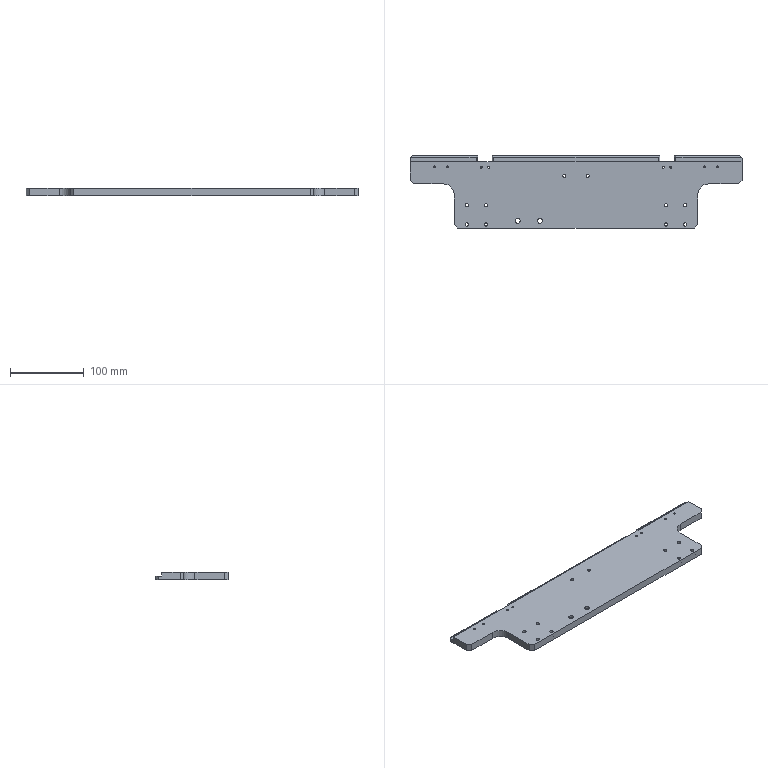Part | NX | 1 solid | 83 faces | box 450 x 98 x 10 mm | volume 340377 mm3 | plane 47 | cylinder 36 | commonest cylinder face diameters 2.5 x8 4.5 x8 8 x8 6 x4 4.2 x2 6.6 x2